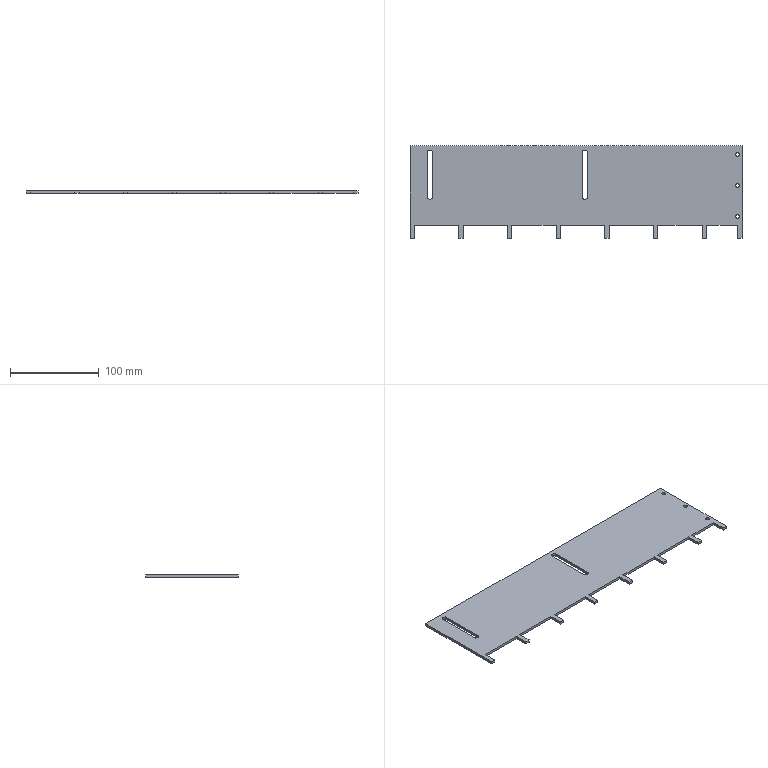Part | SolidWorks | features HoleWzd 2, Cut 1, FlatPattern 1, SMBaseFlange 1, SheetMetal 1 | 1 solid | 48 faces | box 375 x 105 x 3 mm | volume 101027 mm3 | plane 38 | cylinder 10 | commonest cylinder face diameters 4.2 x6 5.8 x4
STEP:
#1=CARTESIAN_POINT('',(372.1,60.,0.));
#2=VERTEX_POINT('',#1);
#3=CARTESIAN_POINT('',(367.9,60.,0.));
#4=VERTEX_POINT('',#3);
#5=CARTESIAN_POINT('',(370.,60.,0.));
#6=DIRECTION('',(0.,0.,-1.));
#7=DIRECTION('',(-1.,0.,0.));
#8=AXIS2_PLACEMENT_3D('',#5,#6,#7);
#9=CIRCLE('',#8,2.1);
#10=EDGE_CURVE('',#2,#4,#9,.T.);
#11=ORIENTED_EDGE('',*,*,#10,.F.);
#12=CARTESIAN_POINT('',(372.1,60.,-3.));
#13=VERTEX_POINT('',#12);
#14=CARTESIAN_POINT('',(372.1,60.,-3.));
#15=DIRECTION('',(0.,0.,-1.));
#16=VECTOR('',#15,1000.);
#17=LINE('',#14,#16);
#18=EDGE_CURVE('',#2,#13,#17,.T.);
#19=ORIENTED_EDGE('',*,*,#18,.T.);
#20=CARTESIAN_POINT('',(367.9,60.,-3.));
#21=VERTEX_POINT('',#20);
#22=CARTESIAN_POINT('',(370.,60.,-3.));
#23=DIRECTION('',(0.,0.,-1.));
#24=DIRECTION('',(-1.,0.,0.));
#25=AXIS2_PLACEMENT_3D('',#22,#23,#24);
#26=CIRCLE('',#25,2.1);
#27=EDGE_CURVE('',#13,#21,#26,.T.);
#28=ORIENTED_EDGE('',*,*,#27,.T.);
#29=CARTESIAN_POINT('',(367.9,60.,-3.));
#30=DIRECTION('',(0.,0.,-1.));
#31=VECTOR('',#30,1000.);
#32=LINE('',#29,#31);
#33=EDGE_CURVE('',#4,#21,#32,.T.);
#34=ORIENTED_EDGE('',*,*,#33,.F.);
#35=EDGE_LOOP('',(#11,#19,#28,#34));
#36=FACE_OUTER_BOUND('',#35,.T.);
#37=CARTESIAN_POINT('',(370.,60.,-3.));
#38=DIRECTION('',(0.,0.,-1.));
#39=DIRECTION('',(-1.,0.,0.));
#40=AXIS2_PLACEMENT_3D('',#37,#38,#39);
#41=CYLINDRICAL_SURFACE('',#40,2.1);
#42=ADVANCED_FACE('',(#36),#41,.F.);
#43=CARTESIAN_POINT('',(372.1,95.,0.));
#44=VERTEX_POINT('',#43);
#45=CARTESIAN_POINT('',(367.9,95.,0.));
#46=VERTEX_POINT('',#45);
#47=CARTESIAN_POINT('',(370.,95.,0.));
#48=DIRECTION('',(0.,0.,-1.));
#49=DIRECTION('',(-1.,0.,0.));
#50=AXIS2_PLACEMENT_3D('',#47,#48,#49);
#51=CIRCLE('',#50,2.1);
#52=EDGE_CURVE('',#44,#46,#51,.T.);
#53=ORIENTED_EDGE('',*,*,#52,.F.);
#54=CARTESIAN_POINT('',(372.1,95.,-3.));
#55=VERTEX_POINT('',#54);
#56=CARTESIAN_POINT('',(372.1,95.,-3.));
#57=DIRECTION('',(0.,0.,-1.));
#58=VECTOR('',#57,1000.);
#59=LINE('',#56,#58);
#60=EDGE_CURVE('',#44,#55,#59,.T.);
#61=ORIENTED_EDGE('',*,*,#60,.T.);
#62=CARTESIAN_POINT('',(367.9,95.,-3.));
#63=VERTEX_POINT('',#62);
#64=CARTESIAN_POINT('',(370.,95.,-3.));
#65=DIRECTION('',(0.,0.,-1.));
#66=DIRECTION('',(-1.,0.,0.));
#67=AXIS2_PLACEMENT_3D('',#64,#65,#66);
#68=CIRCLE('',#67,2.1);
#69=EDGE_CURVE('',#55,#63,#68,.T.);
#70=ORIENTED_EDGE('',*,*,#69,.T.);
#71=CARTESIAN_POINT('',(367.9,95.,-3.));
#72=DIRECTION('',(0.,0.,-1.));
#73=VECTOR('',#72,1000.);
#74=LINE('',#71,#73);
#75=EDGE_CURVE('',#46,#63,#74,.T.);
#76=ORIENTED_EDGE('',*,*,#75,.F.);
#77=EDGE_LOOP('',(#53,#61,#70,#76));
#78=FACE_OUTER_BOUND('',#77,.T.);
#79=CARTESIAN_POINT('',(370.,95.,-3.));
#80=DIRECTION('',(0.,0.,-1.));
#81=DIRECTION('',(-1.,0.,0.));
#82=AXIS2_PLACEMENT_3D('',#79,#80,#81);
#83=CYLINDRICAL_SURFACE('',#82,2.1);
#84=ADVANCED_FACE('',(#78),#83,.F.);
#85=CARTESIAN_POINT('',(372.1,25.,0.));
#86=VERTEX_POINT('',#85);
#87=CARTESIAN_POINT('',(367.9,25.,0.));
#88=VERTEX_POINT('',#87);
#89=CARTESIAN_POINT('',(370.,25.,0.));
#90=DIRECTION('',(0.,0.,-1.));
#91=DIRECTION('',(-1.,0.,0.));
#92=AXIS2_PLACEMENT_3D('',#89,#90,#91);
#93=CIRCLE('',#92,2.1);
#94=EDGE_CURVE('',#86,#88,#93,.T.);
#95=ORIENTED_EDGE('',*,*,#94,.F.);
#96=CARTESIAN_POINT('',(372.1,25.,-3.));
#97=VERTEX_POINT('',#96);
#98=CARTESIAN_POINT('',(372.1,25.,-3.));
#99=DIRECTION('',(0.,0.,-1.));
#100=VECTOR('',#99,1000.);
#101=LINE('',#98,#100);
#102=EDGE_CURVE('',#86,#97,#101,.T.);
#103=ORIENTED_EDGE('',*,*,#102,.T.);
#104=CARTESIAN_POINT('',(367.9,25.,-3.));
#105=VERTEX_POINT('',#104);
#106=CARTESIAN_POINT('',(370.,25.,-3.));
#107=DIRECTION('',(0.,0.,-1.));
#108=DIRECTION('',(-1.,0.,0.));
#109=AXIS2_PLACEMENT_3D('',#106,#107,#108);
#110=CIRCLE('',#109,2.1);
#111=EDGE_CURVE('',#97,#105,#110,.T.);
#112=ORIENTED_EDGE('',*,*,#111,.T.);
#113=CARTESIAN_POINT('',(367.9,25.,-3.));
#114=DIRECTION('',(0.,0.,-1.));
#115=VECTOR('',#114,1000.);
#116=LINE('',#113,#115);
#117=EDGE_CURVE('',#88,#105,#116,.T.);
#118=ORIENTED_EDGE('',*,*,#117,.F.);
#119=EDGE_LOOP('',(#95,#103,#112,#118));
#120=FACE_OUTER_BOUND('',#119,.T.);
#121=CARTESIAN_POINT('',(370.,25.,-3.));
#122=DIRECTION('',(0.,0.,-1.));
#123=DIRECTION('',(-1.,0.,0.));
#124=AXIS2_PLACEMENT_3D('',#121,#122,#123);
#125=CYLINDRICAL_SURFACE('',#124,2.1);
#126=ADVANCED_FACE('',(#120),#125,.F.);
#127=CARTESIAN_POINT('',(5.,0.,-3.));
#128=VERTEX_POINT('',#127);
#129=CARTESIAN_POINT('',(5.,0.,0.));
#130=VERTEX_POINT('',#129);
#131=CARTESIAN_POINT('',(5.,0.,-3.));
#132=DIRECTION('',(0.,0.,1.));
#133=VECTOR('',#132,1000.);
#134=LINE('',#131,#133);
#135=EDGE_CURVE('',#128,#130,#134,.T.);
#136=ORIENTED_EDGE('',*,*,#135,.T.);
#137=CARTESIAN_POINT('',(0.,0.,0.));
#138=VERTEX_POINT('',#137);
#139=CARTESIAN_POINT('',(0.,0.,0.));
#140=DIRECTION('',(1.,0.,0.));
#141=VECTOR('',#140,1000.);
#142=LINE('',#139,#141);
#143=EDGE_CURVE('',#138,#130,#142,.T.);
#144=ORIENTED_EDGE('',*,*,#143,.F.);
#145=CARTESIAN_POINT('',(0.,0.,-3.));
#146=VERTEX_POINT('',#145);
#147=CARTESIAN_POINT('',(0.,0.,-3.));
#148=DIRECTION('',(0.,0.,1.));
#149=VECTOR('',#148,1000.);
#150=LINE('',#147,#149);
#151=EDGE_CURVE('',#146,#138,#150,.T.);
#152=ORIENTED_EDGE('',*,*,#151,.F.);
#153=CARTESIAN_POINT('',(0.,0.,-3.));
#154=DIRECTION('',(1.,0.,0.));
#155=VECTOR('',#154,1000.);
#156=LINE('',#153,#155);
#157=EDGE_CURVE('',#146,#128,#156,.T.);
#158=ORIENTED_EDGE('',*,*,#157,.T.);
#159=EDGE_LOOP('',(#136,#144,#152,#158));
#160=FACE_OUTER_BOUND('',#159,.T.);
#161=CARTESIAN_POINT('',(0.,0.,-3.));
#162=DIRECTION('',(0.,-1.,0.));
#163=DIRECTION('',(0.,0.,-1.));
#164=AXIS2_PLACEMENT_3D('',#161,#162,#163);
#165=PLANE('',#164);
#166=ADVANCED_FACE('',(#160),#165,.T.);
#167=CARTESIAN_POINT('',(280.,0.,-3.));
#168=VERTEX_POINT('',#167);
#169=CARTESIAN_POINT('',(280.,0.,0.));
#170=VERTEX_POINT('',#169);
#171=CARTESIAN_POINT('',(280.,0.,-3.));
#172=DIRECTION('',(0.,0.,1.));
#173=VECTOR('',#172,1000.);
#174=LINE('',#171,#173);
#175=EDGE_CURVE('',#168,#170,#174,.T.);
#176=ORIENTED_EDGE('',*,*,#175,.T.);
#177=CARTESIAN_POINT('',(275.,0.,0.));
#178=VERTEX_POINT('',#177);
#179=CARTESIAN_POINT('',(0.,0.,0.));
#180=DIRECTION('',(1.,0.,0.));
#181=VECTOR('',#180,1000.);
#182=LINE('',#179,#181);
#183=EDGE_CURVE('',#178,#170,#182,.T.);
#184=ORIENTED_EDGE('',*,*,#183,.F.);
#185=CARTESIAN_POINT('',(275.,0.,-3.));
#186=VERTEX_POINT('',#185);
#187=CARTESIAN_POINT('',(275.,0.,-3.));
#188=DIRECTION('',(0.,0.,1.));
#189=VECTOR('',#188,1000.);
#190=LINE('',#187,#189);
#191=EDGE_CURVE('',#186,#178,#190,.T.);
#192=ORIENTED_EDGE('',*,*,#191,.F.);
#193=CARTESIAN_POINT('',(0.,0.,-3.));
#194=DIRECTION('',(1.,0.,0.));
#195=VECTOR('',#194,1000.);
#196=LINE('',#193,#195);
#197=EDGE_CURVE('',#186,#168,#196,.T.);
#198=ORIENTED_EDGE('',*,*,#197,.T.);
#199=EDGE_LOOP('',(#176,#184,#192,#198));
#200=FACE_OUTER_BOUND('',#199,.T.);
#201=CARTESIAN_POINT('',(0.,0.,-3.));
#202=DIRECTION('',(0.,-1.,0.));
#203=DIRECTION('',(0.,0.,-1.));
#204=AXIS2_PLACEMENT_3D('',#201,#202,#203);
#205=PLANE('',#204);
#206=ADVANCED_FACE('',(#200),#205,.T.);
#207=CARTESIAN_POINT('',(225.,0.,-3.));
#208=VERTEX_POINT('',#207);
#209=CARTESIAN_POINT('',(225.,0.,0.));
#210=VERTEX_POINT('',#209);
#211=CARTESIAN_POINT('',(225.,0.,-3.));
#212=DIRECTION('',(0.,0.,1.));
#213=VECTOR('',#212,1000.);
#214=LINE('',#211,#213);
#215=EDGE_CURVE('',#208,#210,#214,.T.);
#216=ORIENTED_EDGE('',*,*,#215,.T.);
#217=CARTESIAN_POINT('',(220.,0.,0.));
#218=VERTEX_POINT('',#217);
#219=CARTESIAN_POINT('',(0.,0.,0.));
#220=DIRECTION('',(1.,0.,0.));
#221=VECTOR('',#220,1000.);
#222=LINE('',#219,#221);
#223=EDGE_CURVE('',#218,#210,#222,.T.);
#224=ORIENTED_EDGE('',*,*,#223,.F.);
#225=CARTESIAN_POINT('',(220.,0.,-3.));
#226=VERTEX_POINT('',#225);
#227=CARTESIAN_POINT('',(220.,0.,-3.));
#228=DIRECTION('',(0.,0.,1.));
#229=VECTOR('',#228,1000.);
#230=LINE('',#227,#229);
#231=EDGE_CURVE('',#226,#218,#230,.T.);
#232=ORIENTED_EDGE('',*,*,#231,.F.);
#233=CARTESIAN_POINT('',(0.,0.,-3.));
#234=DIRECTION('',(1.,0.,0.));
#235=VECTOR('',#234,1000.);
#236=LINE('',#233,#235);
#237=EDGE_CURVE('',#226,#208,#236,.T.);
#238=ORIENTED_EDGE('',*,*,#237,.T.);
#239=EDGE_LOOP('',(#216,#224,#232,#238));
#240=FACE_OUTER_BOUND('',#239,.T.);
#241=CARTESIAN_POINT('',(0.,0.,-3.));
#242=DIRECTION('',(0.,-1.,0.));
#243=DIRECTION('',(0.,0.,-1.));
#244=AXIS2_PLACEMENT_3D('',#241,#242,#243);
#245=PLANE('',#244);
#246=ADVANCED_FACE('',(#240),#245,.T.);
#247=CARTESIAN_POINT('',(330.,0.,-3.));
#248=VERTEX_POINT('',#247);
#249=CARTESIAN_POINT('',(330.,0.,0.));
#250=VERTEX_POINT('',#249);
#251=CARTESIAN_POINT('',(330.,0.,-3.));
#252=DIRECTION('',(0.,0.,1.));
#253=VECTOR('',#252,1000.);
#254=LINE('',#251,#253);
#255=EDGE_CURVE('',#248,#250,#254,.T.);
#256=ORIENTED_EDGE('',*,*,#255,.F.);
#257=CARTESIAN_POINT('',(335.,0.,-3.));
#258=VERTEX_POINT('',#257);
#259=CARTESIAN_POINT('',(0.,0.,-3.));
#260=DIRECTION('',(1.,0.,0.));
#261=VECTOR('',#260,1000.);
#262=LINE('',#259,#261);
#263=EDGE_CURVE('',#248,#258,#262,.T.);
#264=ORIENTED_EDGE('',*,*,#263,.T.);
#265=CARTESIAN_POINT('',(335.,0.,0.));
#266=VERTEX_POINT('',#265);
#267=CARTESIAN_POINT('',(335.,0.,-3.));
#268=DIRECTION('',(0.,0.,1.));
#269=VECTOR('',#268,1000.);
#270=LINE('',#267,#269);
#271=EDGE_CURVE('',#258,#266,#270,.T.);
#272=ORIENTED_EDGE('',*,*,#271,.T.);
#273=CARTESIAN_POINT('',(0.,0.,0.));
#274=DIRECTION('',(1.,0.,0.));
#275=VECTOR('',#274,1000.);
#276=LINE('',#273,#275);
#277=EDGE_CURVE('',#250,#266,#276,.T.);
#278=ORIENTED_EDGE('',*,*,#277,.F.);
#279=EDGE_LOOP('',(#256,#264,#272,#278));
#280=FACE_OUTER_BOUND('',#279,.T.);
#281=CARTESIAN_POINT('',(0.,0.,-3.));
#282=DIRECTION('',(0.,-1.,0.));
#283=DIRECTION('',(0.,0.,-1.));
#284=AXIS2_PLACEMENT_3D('',#281,#282,#283);
#285=PLANE('',#284);
#286=ADVANCED_FACE('',(#280),#285,.T.);
#287=CARTESIAN_POINT('',(55.,0.,-3.));
#288=VERTEX_POINT('',#287);
#289=CARTESIAN_POINT('',(55.,0.,0.));
#290=VERTEX_POINT('',#289);
#291=CARTESIAN_POINT('',(55.,0.,-3.));
#292=DIRECTION('',(0.,0.,1.));
#293=VECTOR('',#292,1000.);
#294=LINE('',#291,#293);
#295=EDGE_CURVE('',#288,#290,#294,.T.);
#296=ORIENTED_EDGE('',*,*,#295,.F.);
#297=CARTESIAN_POINT('',(60.,0.,-3.));
#298=VERTEX_POINT('',#297);
#299=CARTESIAN_POINT('',(0.,0.,-3.));
#300=DIRECTION('',(1.,0.,0.));
#301=VECTOR('',#300,1000.);
#302=LINE('',#299,#301);
#303=EDGE_CURVE('',#288,#298,#302,.T.);
#304=ORIENTED_EDGE('',*,*,#303,.T.);
#305=CARTESIAN_POINT('',(60.,0.,0.));
#306=VERTEX_POINT('',#305);
#307=CARTESIAN_POINT('',(60.,0.,-3.));
#308=DIRECTION('',(0.,0.,1.));
#309=VECTOR('',#308,1000.);
#310=LINE('',#307,#309);
#311=EDGE_CURVE('',#298,#306,#310,.T.);
#312=ORIENTED_EDGE('',*,*,#311,.T.);
#313=CARTESIAN_POINT('',(0.,0.,0.));
#314=DIRECTION('',(1.,0.,0.));
#315=VECTOR('',#314,1000.);
#316=LINE('',#313,#315);
#317=EDGE_CURVE('',#290,#306,#316,.T.);
#318=ORIENTED_EDGE('',*,*,#317,.F.);
#319=EDGE_LOOP('',(#296,#304,#312,#318));
#320=FACE_OUTER_BOUND('',#319,.T.);
#321=CARTESIAN_POINT('',(0.,0.,-3.));
#322=DIRECTION('',(0.,-1.,0.));
#323=DIRECTION('',(0.,0.,-1.));
#324=AXIS2_PLACEMENT_3D('',#321,#322,#323);
#325=PLANE('',#324);
#326=ADVANCED_FACE('',(#320),#325,.T.);
#327=CARTESIAN_POINT('',(110.,0.,-3.));
#328=VERTEX_POINT('',#327);
#329=CARTESIAN_POINT('',(110.,0.,0.));
#330=VERTEX_POINT('',#329);
#331=CARTESIAN_POINT('',(110.,0.,-3.));
#332=DIRECTION('',(0.,0.,1.));
#333=VECTOR('',#332,1000.);
#334=LINE('',#331,#333);
#335=EDGE_CURVE('',#328,#330,#334,.T.);
#336=ORIENTED_EDGE('',*,*,#335,.F.);
#337=CARTESIAN_POINT('',(115.,0.,-3.));
#338=VERTEX_POINT('',#337);
#339=CARTESIAN_POINT('',(0.,0.,-3.));
#340=DIRECTION('',(1.,0.,0.));
#341=VECTOR('',#340,1000.);
#342=LINE('',#339,#341);
#343=EDGE_CURVE('',#328,#338,#342,.T.);
#344=ORIENTED_EDGE('',*,*,#343,.T.);
#345=CARTESIAN_POINT('',(115.,0.,0.));
#346=VERTEX_POINT('',#345);
#347=CARTESIAN_POINT('',(115.,0.,-3.));
#348=DIRECTION('',(0.,0.,1.));
#349=VECTOR('',#348,1000.);
#350=LINE('',#347,#349);
#351=EDGE_CURVE('',#338,#346,#350,.T.);
#352=ORIENTED_EDGE('',*,*,#351,.T.);
#353=CARTESIAN_POINT('',(0.,0.,0.));
#354=DIRECTION('',(1.,0.,0.));
#355=VECTOR('',#354,1000.);
#356=LINE('',#353,#355);
#357=EDGE_CURVE('',#330,#346,#356,.T.);
#358=ORIENTED_EDGE('',*,*,#357,.F.);
#359=EDGE_LOOP('',(#336,#344,#352,#358));
#360=FACE_OUTER_BOUND('',#359,.T.);
#361=CARTESIAN_POINT('',(0.,0.,-3.));
#362=DIRECTION('',(0.,-1.,0.));
#363=DIRECTION('',(0.,0.,-1.));
#364=AXIS2_PLACEMENT_3D('',#361,#362,#363);
#365=PLANE('',#364);
#366=ADVANCED_FACE('',(#360),#365,.T.);
#367=CARTESIAN_POINT('',(165.,0.,-3.));
#368=VERTEX_POINT('',#367);
#369=CARTESIAN_POINT('',(165.,0.,0.));
#370=VERTEX_POINT('',#369);
#371=CARTESIAN_POINT('',(165.,0.,-3.));
#372=DIRECTION('',(0.,0.,1.));
#373=VECTOR('',#372,1000.);
#374=LINE('',#371,#373);
#375=EDGE_CURVE('',#368,#370,#374,.T.);
#376=ORIENTED_EDGE('',*,*,#375,.F.);
#377=CARTESIAN_POINT('',(170.,0.,-3.));
#378=VERTEX_POINT('',#377);
#379=CARTESIAN_POINT('',(0.,0.,-3.));
#380=DIRECTION('',(1.,0.,0.));
#381=VECTOR('',#380,1000.);
#382=LINE('',#379,#381);
#383=EDGE_CURVE('',#368,#378,#382,.T.);
#384=ORIENTED_EDGE('',*,*,#383,.T.);
#385=CARTESIAN_POINT('',(170.,0.,0.));
#386=VERTEX_POINT('',#385);
#387=CARTESIAN_POINT('',(170.,0.,-3.));
#388=DIRECTION('',(0.,0.,1.));
#389=VECTOR('',#388,1000.);
#390=LINE('',#387,#389);
#391=EDGE_CURVE('',#378,#386,#390,.T.);
#392=ORIENTED_EDGE('',*,*,#391,.T.);
#393=CARTESIAN_POINT('',(0.,0.,0.));
#394=DIRECTION('',(1.,0.,0.));
#395=VECTOR('',#394,1000.);
#396=LINE('',#393,#395);
#397=EDGE_CURVE('',#370,#386,#396,.T.);
#398=ORIENTED_EDGE('',*,*,#397,.F.);
#399=EDGE_LOOP('',(#376,#384,#392,#398));
#400=FACE_OUTER_BOUND('',#399,.T.);
#401=CARTESIAN_POINT('',(0.,0.,-3.));
#402=DIRECTION('',(0.,-1.,0.));
#403=DIRECTION('',(0.,0.,-1.));
#404=AXIS2_PLACEMENT_3D('',#401,#402,#403);
#405=PLANE('',#404);
#406=ADVANCED_FACE('',(#400),#405,.T.);
#407=CARTESIAN_POINT('',(370.,60.,0.));
#408=DIRECTION('',(0.,0.,-1.));
#409=DIRECTION('',(-1.,0.,0.));
#410=AXIS2_PLACEMENT_3D('',#407,#408,#409);
#411=CIRCLE('',#410,2.1);
#412=EDGE_CURVE('',#4,#2,#411,.T.);
#413=ORIENTED_EDGE('',*,*,#412,.T.);
#414=ORIENTED_EDGE('',*,*,#10,.T.);
#415=EDGE_LOOP('',(#413,#414));
#416=FACE_BOUND('',#415,.T.);
#417=CARTESIAN_POINT('',(370.,95.,0.));
#418=DIRECTION('',(0.,0.,-1.));
#419=DIRECTION('',(-1.,0.,0.));
#420=AXIS2_PLACEMENT_3D('',#417,#418,#419);
#421=CIRCLE('',#420,2.1);
#422=EDGE_CURVE('',#46,#44,#421,.T.);
#423=ORIENTED_EDGE('',*,*,#422,.T.);
#424=ORIENTED_EDGE('',*,*,#52,.T.);
#425=EDGE_LOOP('',(#423,#424));
#426=FACE_BOUND('',#425,.T.);
#427=CARTESIAN_POINT('',(370.,25.,0.));
#428=DIRECTION('',(0.,0.,-1.));
#429=DIRECTION('',(-1.,0.,0.));
#430=AXIS2_PLACEMENT_3D('',#427,#428,#429);
#431=CIRCLE('',#430,2.1);
#432=EDGE_CURVE('',#88,#86,#431,.T.);
#433=ORIENTED_EDGE('',*,*,#432,.T.);
#434=ORIENTED_EDGE('',*,*,#94,.T.);
#435=EDGE_LOOP('',(#433,#434));
#436=FACE_BOUND('',#435,.T.);
#437=CARTESIAN_POINT('',(25.4,47.,0.));
#438=VERTEX_POINT('',#437);
#439=CARTESIAN_POINT('',(25.4,97.,0.));
#440=VERTEX_POINT('',#439);
#441=CARTESIAN_POINT('',(25.4,47.,0.));
#442=DIRECTION('',(0.,1.,0.));
#443=VECTOR('',#442,1000.);
#444=LINE('',#441,#443);
#445=EDGE_CURVE('',#438,#440,#444,.T.);
#446=ORIENTED_EDGE('',*,*,#445,.F.);
#447=CARTESIAN_POINT('',(19.6,47.,0.));
#448=VERTEX_POINT('',#447);
#449=CARTESIAN_POINT('',(22.5,47.,0.));
#450=DIRECTION('',(0.,0.,1.));
#451=DIRECTION('',(1.,0.,0.));
#452=AXIS2_PLACEMENT_3D('',#449,#450,#451);
#453=CIRCLE('',#452,2.9);
#454=EDGE_CURVE('',#448,#438,#453,.T.);
#455=ORIENTED_EDGE('',*,*,#454,.F.);
#456=CARTESIAN_POINT('',(19.6,97.,0.));
#457=VERTEX_POINT('',#456);
#458=CARTESIAN_POINT('',(19.6,47.,0.));
#459=DIRECTION('',(0.,1.,0.));
#460=VECTOR('',#459,1000.);
#461=LINE('',#458,#460);
#462=EDGE_CURVE('',#448,#457,#461,.T.);
#463=ORIENTED_EDGE('',*,*,#462,.T.);
#464=CARTESIAN_POINT('',(22.5,97.,0.));
#465=DIRECTION('',(0.,0.,1.));
#466=DIRECTION('',(1.,0.,0.));
#467=AXIS2_PLACEMENT_3D('',#464,#465,#466);
#468=CIRCLE('',#467,2.9);
#469=EDGE_CURVE('',#440,#457,#468,.T.);
#470=ORIENTED_EDGE('',*,*,#469,.F.);
#471=EDGE_LOOP('',(#446,#455,#463,#470));
#472=FACE_BOUND('',#471,.T.);
#473=ORIENTED_EDGE('',*,*,#143,.T.);
#474=CARTESIAN_POINT('',(5.,15.,0.));
#475=VERTEX_POINT('',#474);
#476=CARTESIAN_POINT('',(5.,15.,0.));
#477=DIRECTION('',(0.,-1.,0.));
#478=VECTOR('',#477,1000.);
#479=LINE('',#476,#478);
#480=EDGE_CURVE('',#475,#130,#479,.T.);
#481=ORIENTED_EDGE('',*,*,#480,.F.);
#482=CARTESIAN_POINT('',(55.,15.,0.));
#483=VERTEX_POINT('',#482);
#484=CARTESIAN_POINT('',(5.,15.,0.));
#485=DIRECTION('',(-1.,0.,0.));
#486=VECTOR('',#485,1000.);
#487=LINE('',#484,#486);
#488=EDGE_CURVE('',#483,#475,#487,.T.);
#489=ORIENTED_EDGE('',*,*,#488,.F.);
#490=CARTESIAN_POINT('',(55.,15.,0.));
#491=DIRECTION('',(0.,1.,0.));
#492=VECTOR('',#491,1000.);
#493=LINE('',#490,#492);
#494=EDGE_CURVE('',#290,#483,#493,.T.);
#495=ORIENTED_EDGE('',*,*,#494,.F.);
#496=ORIENTED_EDGE('',*,*,#317,.T.);
#497=CARTESIAN_POINT('',(60.,15.,0.));
#498=VERTEX_POINT('',#497);
#499=CARTESIAN_POINT('',(60.,15.,0.));
#500=DIRECTION('',(0.,-1.,0.));
#501=VECTOR('',#500,1000.);
#502=LINE('',#499,#501);
#503=EDGE_CURVE('',#498,#306,#502,.T.);
#504=ORIENTED_EDGE('',*,*,#503,.F.);
#505=CARTESIAN_POINT('',(110.,15.,0.));
#506=VERTEX_POINT('',#505);
#507=CARTESIAN_POINT('',(60.,15.,0.));
#508=DIRECTION('',(-1.,0.,0.));
#509=VECTOR('',#508,1000.);
#510=LINE('',#507,#509);
#511=EDGE_CURVE('',#506,#498,#510,.T.);
#512=ORIENTED_EDGE('',*,*,#511,.F.);
#513=CARTESIAN_POINT('',(110.,15.,0.));
#514=DIRECTION('',(0.,1.,0.));
#515=VECTOR('',#514,1000.);
#516=LINE('',#513,#515);
#517=EDGE_CURVE('',#330,#506,#516,.T.);
#518=ORIENTED_EDGE('',*,*,#517,.F.);
#519=ORIENTED_EDGE('',*,*,#357,.T.);
#520=CARTESIAN_POINT('',(115.,15.,0.));
#521=VERTEX_POINT('',#520);
#522=CARTESIAN_POINT('',(115.,15.,0.));
#523=DIRECTION('',(0.,-1.,0.));
#524=VECTOR('',#523,1000.);
#525=LINE('',#522,#524);
#526=EDGE_CURVE('',#521,#346,#525,.T.);
#527=ORIENTED_EDGE('',*,*,#526,.F.);
#528=CARTESIAN_POINT('',(165.,15.,0.));
#529=VERTEX_POINT('',#528);
#530=CARTESIAN_POINT('',(115.,15.,0.));
#531=DIRECTION('',(-1.,0.,0.));
#532=VECTOR('',#531,1000.);
#533=LINE('',#530,#532);
#534=EDGE_CURVE('',#529,#521,#533,.T.);
#535=ORIENTED_EDGE('',*,*,#534,.F.);
#536=CARTESIAN_POINT('',(165.,15.,0.));
#537=DIRECTION('',(0.,1.,0.));
#538=VECTOR('',#537,1000.);
#539=LINE('',#536,#538);
#540=EDGE_CURVE('',#370,#529,#539,.T.);
#541=ORIENTED_EDGE('',*,*,#540,.F.);
#542=ORIENTED_EDGE('',*,*,#397,.T.);
#543=CARTESIAN_POINT('',(170.,15.,0.));
#544=VERTEX_POINT('',#543);
#545=CARTESIAN_POINT('',(170.,15.,0.));
#546=DIRECTION('',(0.,-1.,0.));
#547=VECTOR('',#546,1000.);
#548=LINE('',#545,#547);
#549=EDGE_CURVE('',#544,#386,#548,.T.);
#550=ORIENTED_EDGE('',*,*,#549,.F.);
#551=CARTESIAN_POINT('',(220.,15.,0.));
#552=VERTEX_POINT('',#551);
#553=CARTESIAN_POINT('',(170.,15.,0.));
#554=DIRECTION('',(-1.,0.,0.));
#555=VECTOR('',#554,1000.);
#556=LINE('',#553,#555);
#557=EDGE_CURVE('',#552,#544,#556,.T.);
#558=ORIENTED_EDGE('',*,*,#557,.F.);
#559=CARTESIAN_POINT('',(220.,15.,0.));
#560=DIRECTION('',(0.,1.,0.));
#561=VECTOR('',#560,1000.);
#562=LINE('',#559,#561);
#563=EDGE_CURVE('',#218,#552,#562,.T.);
#564=ORIENTED_EDGE('',*,*,#563,.F.);
#565=ORIENTED_EDGE('',*,*,#223,.T.);
#566=CARTESIAN_POINT('',(225.,15.,0.));
#567=VERTEX_POINT('',#566);
#568=CARTESIAN_POINT('',(225.,15.,0.));
#569=DIRECTION('',(0.,-1.,0.));
#570=VECTOR('',#569,1000.);
#571=LINE('',#568,#570);
#572=EDGE_CURVE('',#567,#210,#571,.T.);
#573=ORIENTED_EDGE('',*,*,#572,.F.);
#574=CARTESIAN_POINT('',(275.,15.,0.));
#575=VERTEX_POINT('',#574);
#576=CARTESIAN_POINT('',(225.,15.,0.));
#577=DIRECTION('',(-1.,0.,0.));
#578=VECTOR('',#577,1000.);
#579=LINE('',#576,#578);
#580=EDGE_CURVE('',#575,#567,#579,.T.);
#581=ORIENTED_EDGE('',*,*,#580,.F.);
#582=CARTESIAN_POINT('',(275.,15.,0.));
#583=DIRECTION('',(0.,1.,0.));
#584=VECTOR('',#583,1000.);
#585=LINE('',#582,#584);
#586=EDGE_CURVE('',#178,#575,#585,.T.);
#587=ORIENTED_EDGE('',*,*,#586,.F.);
#588=ORIENTED_EDGE('',*,*,#183,.T.);
#589=CARTESIAN_POINT('',(280.,15.,0.));
#590=VERTEX_POINT('',#589);
#591=CARTESIAN_POINT('',(280.,15.,0.));
#592=DIRECTION('',(0.,-1.,0.));
#593=VECTOR('',#592,1000.);
#594=LINE('',#591,#593);
#595=EDGE_CURVE('',#590,#170,#594,.T.);
#596=ORIENTED_EDGE('',*,*,#595,.F.);
#597=CARTESIAN_POINT('',(330.,15.,0.));
#598=VERTEX_POINT('',#597);
#599=CARTESIAN_POINT('',(280.,15.,0.));
#600=DIRECTION('',(-1.,0.,0.));
#601=VECTOR('',#600,1000.);
#602=LINE('',#599,#601);
#603=EDGE_CURVE('',#598,#590,#602,.T.);
#604=ORIENTED_EDGE('',*,*,#603,.F.);
#605=CARTESIAN_POINT('',(330.,15.,0.));
#606=DIRECTION('',(0.,1.,0.));
#607=VECTOR('',#606,1000.);
#608=LINE('',#605,#607);
#609=EDGE_CURVE('',#250,#598,#608,.T.);
#610=ORIENTED_EDGE('',*,*,#609,.F.);
#611=ORIENTED_EDGE('',*,*,#277,.T.);
#612=CARTESIAN_POINT('',(335.,15.,0.));
#613=VERTEX_POINT('',#612);
#614=CARTESIAN_POINT('',(335.,15.,0.));
#615=DIRECTION('',(0.,-1.,0.));
#616=VECTOR('',#615,1000.);
#617=LINE('',#614,#616);
#618=EDGE_CURVE('',#613,#266,#617,.T.);
#619=ORIENTED_EDGE('',*,*,#618,.F.);
#620=CARTESIAN_POINT('',(370.,15.,0.));
#621=VERTEX_POINT('',#620);
#622=CARTESIAN_POINT('',(335.,15.,0.));
#623=DIRECTION('',(-1.,0.,0.));
#624=VECTOR('',#623,1000.);
#625=LINE('',#622,#624);
#626=EDGE_CURVE('',#621,#613,#625,.T.);
#627=ORIENTED_EDGE('',*,*,#626,.F.);
#628=CARTESIAN_POINT('',(370.,0.,0.));
#629=VERTEX_POINT('',#628);
#630=CARTESIAN_POINT('',(370.,15.,0.));
#631=DIRECTION('',(0.,1.,0.));
#632=VECTOR('',#631,1000.);
#633=LINE('',#630,#632);
#634=EDGE_CURVE('',#629,#621,#633,.T.);
#635=ORIENTED_EDGE('',*,*,#634,.F.);
#636=CARTESIAN_POINT('',(375.,0.,0.));
#637=VERTEX_POINT('',#636);
#638=CARTESIAN_POINT('',(0.,0.,0.));
#639=DIRECTION('',(1.,0.,0.));
#640=VECTOR('',#639,1000.);
#641=LINE('',#638,#640);
#642=EDGE_CURVE('',#629,#637,#641,.T.);
#643=ORIENTED_EDGE('',*,*,#642,.T.);
#644=CARTESIAN_POINT('',(375.,105.,0.));
#645=VERTEX_POINT('',#644);
#646=CARTESIAN_POINT('',(375.,0.,0.));
#647=DIRECTION('',(0.,1.,0.));
#648=VECTOR('',#647,1000.);
#649=LINE('',#646,#648);
#650=EDGE_CURVE('',#637,#645,#649,.T.);
#651=ORIENTED_EDGE('',*,*,#650,.T.);
#652=CARTESIAN_POINT('',(0.,105.,0.));
#653=VERTEX_POINT('',#652);
#654=CARTESIAN_POINT('',(0.,105.,0.));
#655=DIRECTION('',(-1.,0.,0.));
#656=VECTOR('',#655,1000.);
#657=LINE('',#654,#656);
#658=EDGE_CURVE('',#645,#653,#657,.T.);
#659=ORIENTED_EDGE('',*,*,#658,.T.);
#660=CARTESIAN_POINT('',(0.,0.,0.));
#661=DIRECTION('',(0.,-1.,0.));
#662=VECTOR('',#661,1000.);
#663=LINE('',#660,#662);
#664=EDGE_CURVE('',#653,#138,#663,.T.);
#665=ORIENTED_EDGE('',*,*,#664,.T.);
#666=EDGE_LOOP('',(#473,#481,#489,#495,#496,#504,#512,#518,#519,#527,#535,#541,#542,#550,#558,#564,#565,#573,#581,#587,#588,#596,#604,#610,#611,#619,#627,#635,#643,#651,#659,#665));
#667=FACE_OUTER_BOUND('',#666,.T.);
#668=CARTESIAN_POINT('',(200.4,47.,0.));
#669=VERTEX_POINT('',#668);
#670=CARTESIAN_POINT('',(200.4,97.,0.));
#671=VERTEX_POINT('',#670);
#672=CARTESIAN_POINT('',(200.4,47.,0.));
#673=DIRECTION('',(0.,1.,0.));
#674=VECTOR('',#673,1000.);
#675=LINE('',#672,#674);
#676=EDGE_CURVE('',#669,#671,#675,.T.);
#677=ORIENTED_EDGE('',*,*,#676,.F.);
#678=CARTESIAN_POINT('',(194.6,47.,0.));
#679=VERTEX_POINT('',#678);
#680=CARTESIAN_POINT('',(197.5,47.,0.));
#681=DIRECTION('',(0.,0.,1.));
#682=DIRECTION('',(1.,0.,0.));
#683=AXIS2_PLACEMENT_3D('',#680,#681,#682);
#684=CIRCLE('',#683,2.9);
#685=EDGE_CURVE('',#679,#669,#684,.T.);
#686=ORIENTED_EDGE('',*,*,#685,.F.);
#687=CARTESIAN_POINT('',(194.6,97.,0.));
#688=VERTEX_POINT('',#687);
#689=CARTESIAN_POINT('',(194.6,47.,0.));
#690=DIRECTION('',(0.,1.,0.));
#691=VECTOR('',#690,1000.);
#692=LINE('',#689,#691);
#693=EDGE_CURVE('',#679,#688,#692,.T.);
#694=ORIENTED_EDGE('',*,*,#693,.T.);
#695=CARTESIAN_POINT('',(197.5,97.,0.));
#696=DIRECTION('',(0.,0.,1.));
#697=DIRECTION('',(1.,0.,0.));
#698=AXIS2_PLACEMENT_3D('',#695,#696,#697);
#699=CIRCLE('',#698,2.9);
#700=EDGE_CURVE('',#671,#688,#699,.T.);
#701=ORIENTED_EDGE('',*,*,#700,.F.);
#702=EDGE_LOOP('',(#677,#686,#694,#701));
#703=FACE_BOUND('',#702,.T.);
#704=CARTESIAN_POINT('',(0.,0.,0.));
#705=DIRECTION('',(0.,0.,-1.));
#706=DIRECTION('',(-1.,0.,0.));
#707=AXIS2_PLACEMENT_3D('',#704,#705,#706);
#708=PLANE('',#707);
#709=ADVANCED_FACE('',(#416,#426,#436,#472,#667,#703),#708,.F.);
#710=ORIENTED_EDGE('',*,*,#664,.F.);
#711=CARTESIAN_POINT('',(0.,105.,-3.));
#712=VERTEX_POINT('',#711);
#713=CARTESIAN_POINT('',(0.,105.,-3.));
#714=DIRECTION('',(0.,0.,1.));
#715=VECTOR('',#714,1000.);
#716=LINE('',#713,#715);
#717=EDGE_CURVE('',#712,#653,#716,.T.);
#718=ORIENTED_EDGE('',*,*,#717,.F.);
#719=CARTESIAN_POINT('',(0.,0.,-3.));
#720=DIRECTION('',(0.,-1.,0.));
#721=VECTOR('',#720,1000.);
#722=LINE('',#719,#721);
#723=EDGE_CURVE('',#712,#146,#722,.T.);
#724=ORIENTED_EDGE('',*,*,#723,.T.);
#725=ORIENTED_EDGE('',*,*,#151,.T.);
#726=EDGE_LOOP('',(#710,#718,#724,#725));
#727=FACE_OUTER_BOUND('',#726,.T.);
#728=CARTESIAN_POINT('',(0.,0.,-3.));
#729=DIRECTION('',(-1.,0.,0.));
#730=DIRECTION('',(0.,0.,1.));
#731=AXIS2_PLACEMENT_3D('',#728,#729,#730);
#732=PLANE('',#731);
#733=ADVANCED_FACE('',(#727),#732,.T.);
#734=ORIENTED_EDGE('',*,*,#658,.F.);
#735=CARTESIAN_POINT('',(375.,105.,-3.));
#736=VERTEX_POINT('',#735);
#737=CARTESIAN_POINT('',(375.,105.,-3.));
#738=DIRECTION('',(0.,0.,1.));
#739=VECTOR('',#738,1000.);
#740=LINE('',#737,#739);
#741=EDGE_CURVE('',#736,#645,#740,.T.);
#742=ORIENTED_EDGE('',*,*,#741,.F.);
#743=CARTESIAN_POINT('',(0.,105.,-3.));
#744=DIRECTION('',(-1.,0.,0.));
#745=VECTOR('',#744,1000.);
#746=LINE('',#743,#745);
#747=EDGE_CURVE('',#736,#712,#746,.T.);
#748=ORIENTED_EDGE('',*,*,#747,.T.);
#749=ORIENTED_EDGE('',*,*,#717,.T.);
#750=EDGE_LOOP('',(#734,#742,#748,#749));
#751=FACE_OUTER_BOUND('',#750,.T.);
#752=CARTESIAN_POINT('',(0.,105.,-3.));
#753=DIRECTION('',(0.,1.,0.));
#754=DIRECTION('',(0.,0.,1.));
#755=AXIS2_PLACEMENT_3D('',#752,#753,#754);
#756=PLANE('',#755);
#757=ADVANCED_FACE('',(#751),#756,.T.);
#758=ORIENTED_EDGE('',*,*,#650,.F.);
#759=CARTESIAN_POINT('',(375.,0.,-3.));
#760=VERTEX_POINT('',#759);
#761=CARTESIAN_POINT('',(375.,0.,-3.));
#762=DIRECTION('',(0.,0.,1.));
#763=VECTOR('',#762,1000.);
#764=LINE('',#761,#763);
#765=EDGE_CURVE('',#760,#637,#764,.T.);
#766=ORIENTED_EDGE('',*,*,#765,.F.);
#767=CARTESIAN_POINT('',(375.,0.,-3.));
#768=DIRECTION('',(0.,1.,0.));
#769=VECTOR('',#768,1000.);
#770=LINE('',#767,#769);
#771=EDGE_CURVE('',#760,#736,#770,.T.);
#772=ORIENTED_EDGE('',*,*,#771,.T.);
#773=ORIENTED_EDGE('',*,*,#741,.T.);
#774=EDGE_LOOP('',(#758,#766,#772,#773));
#775=FACE_OUTER_BOUND('',#774,.T.);
#776=CARTESIAN_POINT('',(375.,0.,-3.));
#777=DIRECTION('',(1.,0.,0.));
#778=DIRECTION('',(0.,0.,-1.));
#779=AXIS2_PLACEMENT_3D('',#776,#777,#778);
#780=PLANE('',#779);
#781=ADVANCED_FACE('',(#775),#780,.T.);
#782=CARTESIAN_POINT('',(370.,0.,-3.));
#783=VERTEX_POINT('',#782);
#784=CARTESIAN_POINT('',(370.,0.,-3.));
#785=DIRECTION('',(0.,0.,1.));
#786=VECTOR('',#785,1000.);
#787=LINE('',#784,#786);
#788=EDGE_CURVE('',#783,#629,#787,.T.);
#789=ORIENTED_EDGE('',*,*,#788,.F.);
#790=CARTESIAN_POINT('',(0.,0.,-3.));
#791=DIRECTION('',(1.,0.,0.));
#792=VECTOR('',#791,1000.);
#793=LINE('',#790,#792);
#794=EDGE_CURVE('',#783,#760,#793,.T.);
#795=ORIENTED_EDGE('',*,*,#794,.T.);
#796=ORIENTED_EDGE('',*,*,#765,.T.);
#797=ORIENTED_EDGE('',*,*,#642,.F.);
#798=EDGE_LOOP('',(#789,#795,#796,#797));
#799=FACE_OUTER_BOUND('',#798,.T.);
#800=CARTESIAN_POINT('',(0.,0.,-3.));
#801=DIRECTION('',(0.,-1.,0.));
#802=DIRECTION('',(0.,0.,-1.));
#803=AXIS2_PLACEMENT_3D('',#800,#801,#802);
#804=PLANE('',#803);
#805=ADVANCED_FACE('',(#799),#804,.T.);
#806=CARTESIAN_POINT('',(370.,60.,-3.));
#807=DIRECTION('',(0.,0.,-1.));
#808=DIRECTION('',(-1.,0.,0.));
#809=AXIS2_PLACEMENT_3D('',#806,#807,#808);
#810=CIRCLE('',#809,2.1);
#811=EDGE_CURVE('',#21,#13,#810,.T.);
#812=ORIENTED_EDGE('',*,*,#811,.F.);
#813=ORIENTED_EDGE('',*,*,#27,.F.);
#814=EDGE_LOOP('',(#812,#813));
#815=FACE_BOUND('',#814,.T.);
#816=CARTESIAN_POINT('',(370.,95.,-3.));
#817=DIRECTION('',(0.,0.,-1.));
#818=DIRECTION('',(-1.,0.,0.));
#819=AXIS2_PLACEMENT_3D('',#816,#817,#818);
#820=CIRCLE('',#819,2.1);
#821=EDGE_CURVE('',#63,#55,#820,.T.);
#822=ORIENTED_EDGE('',*,*,#821,.F.);
#823=ORIENTED_EDGE('',*,*,#69,.F.);
#824=EDGE_LOOP('',(#822,#823));
#825=FACE_BOUND('',#824,.T.);
#826=CARTESIAN_POINT('',(370.,25.,-3.));
#827=DIRECTION('',(0.,0.,-1.));
#828=DIRECTION('',(-1.,0.,0.));
#829=AXIS2_PLACEMENT_3D('',#826,#827,#828);
#830=CIRCLE('',#829,2.1);
#831=EDGE_CURVE('',#105,#97,#830,.T.);
#832=ORIENTED_EDGE('',*,*,#831,.F.);
#833=ORIENTED_EDGE('',*,*,#111,.F.);
#834=EDGE_LOOP('',(#832,#833));
#835=FACE_BOUND('',#834,.T.);
#836=CARTESIAN_POINT('',(5.,15.,-3.));
#837=VERTEX_POINT('',#836);
#838=CARTESIAN_POINT('',(5.,15.,-3.));
#839=DIRECTION('',(0.,-1.,0.));
#840=VECTOR('',#839,1000.);
#841=LINE('',#838,#840);
#842=EDGE_CURVE('',#837,#128,#841,.T.);
#843=ORIENTED_EDGE('',*,*,#842,.T.);
#844=ORIENTED_EDGE('',*,*,#157,.F.);
#845=ORIENTED_EDGE('',*,*,#723,.F.);
#846=ORIENTED_EDGE('',*,*,#747,.F.);
#847=ORIENTED_EDGE('',*,*,#771,.F.);
#848=ORIENTED_EDGE('',*,*,#794,.F.);
#849=CARTESIAN_POINT('',(370.,15.,-3.));
#850=VERTEX_POINT('',#849);
#851=CARTESIAN_POINT('',(370.,15.,-3.));
#852=DIRECTION('',(0.,1.,0.));
#853=VECTOR('',#852,1000.);
#854=LINE('',#851,#853);
#855=EDGE_CURVE('',#783,#850,#854,.T.);
#856=ORIENTED_EDGE('',*,*,#855,.T.);
#857=CARTESIAN_POINT('',(335.,15.,-3.));
#858=VERTEX_POINT('',#857);
#859=CARTESIAN_POINT('',(335.,15.,-3.));
#860=DIRECTION('',(-1.,0.,0.));
#861=VECTOR('',#860,1000.);
#862=LINE('',#859,#861);
#863=EDGE_CURVE('',#850,#858,#862,.T.);
#864=ORIENTED_EDGE('',*,*,#863,.T.);
#865=CARTESIAN_POINT('',(335.,15.,-3.));
#866=DIRECTION('',(0.,-1.,0.));
#867=VECTOR('',#866,1000.);
#868=LINE('',#865,#867);
#869=EDGE_CURVE('',#858,#258,#868,.T.);
#870=ORIENTED_EDGE('',*,*,#869,.T.);
#871=ORIENTED_EDGE('',*,*,#263,.F.);
#872=CARTESIAN_POINT('',(330.,15.,-3.));
#873=VERTEX_POINT('',#872);
#874=CARTESIAN_POINT('',(330.,15.,-3.));
#875=DIRECTION('',(0.,1.,0.));
#876=VECTOR('',#875,1000.);
#877=LINE('',#874,#876);
#878=EDGE_CURVE('',#248,#873,#877,.T.);
#879=ORIENTED_EDGE('',*,*,#878,.T.);
#880=CARTESIAN_POINT('',(280.,15.,-3.));
#881=VERTEX_POINT('',#880);
#882=CARTESIAN_POINT('',(280.,15.,-3.));
#883=DIRECTION('',(-1.,0.,0.));
#884=VECTOR('',#883,1000.);
#885=LINE('',#882,#884);
#886=EDGE_CURVE('',#873,#881,#885,.T.);
#887=ORIENTED_EDGE('',*,*,#886,.T.);
#888=CARTESIAN_POINT('',(280.,15.,-3.));
#889=DIRECTION('',(0.,-1.,0.));
#890=VECTOR('',#889,1000.);
#891=LINE('',#888,#890);
#892=EDGE_CURVE('',#881,#168,#891,.T.);
#893=ORIENTED_EDGE('',*,*,#892,.T.);
#894=ORIENTED_EDGE('',*,*,#197,.F.);
#895=CARTESIAN_POINT('',(275.,15.,-3.));
#896=VERTEX_POINT('',#895);
#897=CARTESIAN_POINT('',(275.,15.,-3.));
#898=DIRECTION('',(0.,1.,0.));
#899=VECTOR('',#898,1000.);
#900=LINE('',#897,#899);
#901=EDGE_CURVE('',#186,#896,#900,.T.);
#902=ORIENTED_EDGE('',*,*,#901,.T.);
#903=CARTESIAN_POINT('',(225.,15.,-3.));
#904=VERTEX_POINT('',#903);
#905=CARTESIAN_POINT('',(225.,15.,-3.));
#906=DIRECTION('',(-1.,0.,0.));
#907=VECTOR('',#906,1000.);
#908=LINE('',#905,#907);
#909=EDGE_CURVE('',#896,#904,#908,.T.);
#910=ORIENTED_EDGE('',*,*,#909,.T.);
#911=CARTESIAN_POINT('',(225.,15.,-3.));
#912=DIRECTION('',(0.,-1.,0.));
#913=VECTOR('',#912,1000.);
#914=LINE('',#911,#913);
#915=EDGE_CURVE('',#904,#208,#914,.T.);
#916=ORIENTED_EDGE('',*,*,#915,.T.);
#917=ORIENTED_EDGE('',*,*,#237,.F.);
#918=CARTESIAN_POINT('',(220.,15.,-3.));
#919=VERTEX_POINT('',#918);
#920=CARTESIAN_POINT('',(220.,15.,-3.));
#921=DIRECTION('',(0.,1.,0.));
#922=VECTOR('',#921,1000.);
#923=LINE('',#920,#922);
#924=EDGE_CURVE('',#226,#919,#923,.T.);
#925=ORIENTED_EDGE('',*,*,#924,.T.);
#926=CARTESIAN_POINT('',(170.,15.,-3.));
#927=VERTEX_POINT('',#926);
#928=CARTESIAN_POINT('',(170.,15.,-3.));
#929=DIRECTION('',(-1.,0.,0.));
#930=VECTOR('',#929,1000.);
#931=LINE('',#928,#930);
#932=EDGE_CURVE('',#919,#927,#931,.T.);
#933=ORIENTED_EDGE('',*,*,#932,.T.);
#934=CARTESIAN_POINT('',(170.,15.,-3.));
#935=DIRECTION('',(0.,-1.,0.));
#936=VECTOR('',#935,1000.);
#937=LINE('',#934,#936);
#938=EDGE_CURVE('',#927,#378,#937,.T.);
#939=ORIENTED_EDGE('',*,*,#938,.T.);
#940=ORIENTED_EDGE('',*,*,#383,.F.);
#941=CARTESIAN_POINT('',(165.,15.,-3.));
#942=VERTEX_POINT('',#941);
#943=CARTESIAN_POINT('',(165.,15.,-3.));
#944=DIRECTION('',(0.,1.,0.));
#945=VECTOR('',#944,1000.);
#946=LINE('',#943,#945);
#947=EDGE_CURVE('',#368,#942,#946,.T.);
#948=ORIENTED_EDGE('',*,*,#947,.T.);
#949=CARTESIAN_POINT('',(115.,15.,-3.));
#950=VERTEX_POINT('',#949);
#951=CARTESIAN_POINT('',(115.,15.,-3.));
#952=DIRECTION('',(-1.,0.,0.));
#953=VECTOR('',#952,1000.);
#954=LINE('',#951,#953);
#955=EDGE_CURVE('',#942,#950,#954,.T.);
#956=ORIENTED_EDGE('',*,*,#955,.T.);
#957=CARTESIAN_POINT('',(115.,15.,-3.));
#958=DIRECTION('',(0.,-1.,0.));
#959=VECTOR('',#958,1000.);
#960=LINE('',#957,#959);
#961=EDGE_CURVE('',#950,#338,#960,.T.);
#962=ORIENTED_EDGE('',*,*,#961,.T.);
#963=ORIENTED_EDGE('',*,*,#343,.F.);
#964=CARTESIAN_POINT('',(110.,15.,-3.));
#965=VERTEX_POINT('',#964);
#966=CARTESIAN_POINT('',(110.,15.,-3.));
#967=DIRECTION('',(0.,1.,0.));
#968=VECTOR('',#967,1000.);
#969=LINE('',#966,#968);
#970=EDGE_CURVE('',#328,#965,#969,.T.);
#971=ORIENTED_EDGE('',*,*,#970,.T.);
#972=CARTESIAN_POINT('',(60.,15.,-3.));
#973=VERTEX_POINT('',#972);
#974=CARTESIAN_POINT('',(60.,15.,-3.));
#975=DIRECTION('',(-1.,0.,0.));
#976=VECTOR('',#975,1000.);
#977=LINE('',#974,#976);
#978=EDGE_CURVE('',#965,#973,#977,.T.);
#979=ORIENTED_EDGE('',*,*,#978,.T.);
#980=CARTESIAN_POINT('',(60.,15.,-3.));
#981=DIRECTION('',(0.,-1.,0.));
#982=VECTOR('',#981,1000.);
#983=LINE('',#980,#982);
#984=EDGE_CURVE('',#973,#298,#983,.T.);
#985=ORIENTED_EDGE('',*,*,#984,.T.);
#986=ORIENTED_EDGE('',*,*,#303,.F.);
#987=CARTESIAN_POINT('',(55.,15.,-3.));
#988=VERTEX_POINT('',#987);
#989=CARTESIAN_POINT('',(55.,15.,-3.));
#990=DIRECTION('',(0.,1.,0.));
#991=VECTOR('',#990,1000.);
#992=LINE('',#989,#991);
#993=EDGE_CURVE('',#288,#988,#992,.T.);
#994=ORIENTED_EDGE('',*,*,#993,.T.);
#995=CARTESIAN_POINT('',(5.,15.,-3.));
#996=DIRECTION('',(-1.,0.,0.));
#997=VECTOR('',#996,1000.);
#998=LINE('',#995,#997);
#999=EDGE_CURVE('',#988,#837,#998,.T.);
#1000=ORIENTED_EDGE('',*,*,#999,.T.);
#1001=EDGE_LOOP('',(#843,#844,#845,#846,#847,#848,#856,#864,#870,#871,#879,#887,#893,#894,#902,#910,#916,#917,#925,#933,#939,#940,#948,#956,#962,#963,#971,#979,#985,#986,#994,#1000));
#1002=FACE_OUTER_BOUND('',#1001,.T.);
#1003=CARTESIAN_POINT('',(194.6,47.,-3.));
#1004=VERTEX_POINT('',#1003);
#1005=CARTESIAN_POINT('',(194.6,97.,-3.));
#1006=VERTEX_POINT('',#1005);
#1007=CARTESIAN_POINT('',(194.6,0.,-3.));
#1008=DIRECTION('',(0.,1.,0.));
#1009=VECTOR('',#1008,1000.);
#1010=LINE('',#1007,#1009);
#1011=EDGE_CURVE('',#1004,#1006,#1010,.T.);
#1012=ORIENTED_EDGE('',*,*,#1011,.F.);
#1013=CARTESIAN_POINT('',(200.4,47.,-3.));
#1014=VERTEX_POINT('',#1013);
#1015=CARTESIAN_POINT('',(197.5,47.,-3.));
#1016=DIRECTION('',(0.,0.,-1.));
#1017=DIRECTION('',(-1.,0.,0.));
#1018=AXIS2_PLACEMENT_3D('',#1015,#1016,#1017);
#1019=CIRCLE('',#1018,2.9);
#1020=EDGE_CURVE('',#1014,#1004,#1019,.T.);
#1021=ORIENTED_EDGE('',*,*,#1020,.F.);
#1022=CARTESIAN_POINT('',(200.4,97.,-3.));
#1023=VERTEX_POINT('',#1022);
#1024=CARTESIAN_POINT('',(200.4,0.,-3.));
#1025=DIRECTION('',(0.,-1.,0.));
#1026=VECTOR('',#1025,1000.);
#1027=LINE('',#1024,#1026);
#1028=EDGE_CURVE('',#1023,#1014,#1027,.T.);
#1029=ORIENTED_EDGE('',*,*,#1028,.F.);
#1030=CARTESIAN_POINT('',(197.5,97.,-3.));
#1031=DIRECTION('',(0.,0.,-1.));
#1032=DIRECTION('',(-1.,0.,0.));
#1033=AXIS2_PLACEMENT_3D('',#1030,#1031,#1032);
#1034=CIRCLE('',#1033,2.9);
#1035=EDGE_CURVE('',#1006,#1023,#1034,.T.);
#1036=ORIENTED_EDGE('',*,*,#1035,.F.);
#1037=EDGE_LOOP('',(#1012,#1021,#1029,#1036));
#1038=FACE_BOUND('',#1037,.T.);
#1039=CARTESIAN_POINT('',(19.6,47.,-3.));
#1040=VERTEX_POINT('',#1039);
#1041=CARTESIAN_POINT('',(19.6,97.,-3.));
#1042=VERTEX_POINT('',#1041);
#1043=CARTESIAN_POINT('',(19.6,0.,-3.));
#1044=DIRECTION('',(0.,1.,0.));
#1045=VECTOR('',#1044,1000.);
#1046=LINE('',#1043,#1045);
#1047=EDGE_CURVE('',#1040,#1042,#1046,.T.);
#1048=ORIENTED_EDGE('',*,*,#1047,.F.);
#1049=CARTESIAN_POINT('',(25.4,47.,-3.));
#1050=VERTEX_POINT('',#1049);
#1051=CARTESIAN_POINT('',(22.5,47.,-3.));
#1052=DIRECTION('',(0.,0.,-1.));
#1053=DIRECTION('',(-1.,0.,0.));
#1054=AXIS2_PLACEMENT_3D('',#1051,#1052,#1053);
#1055=CIRCLE('',#1054,2.9);
#1056=EDGE_CURVE('',#1050,#1040,#1055,.T.);
#1057=ORIENTED_EDGE('',*,*,#1056,.F.);
#1058=CARTESIAN_POINT('',(25.4,97.,-3.));
#1059=VERTEX_POINT('',#1058);
#1060=CARTESIAN_POINT('',(25.4,0.,-3.));
#1061=DIRECTION('',(0.,-1.,0.));
#1062=VECTOR('',#1061,1000.);
#1063=LINE('',#1060,#1062);
#1064=EDGE_CURVE('',#1059,#1050,#1063,.T.);
#1065=ORIENTED_EDGE('',*,*,#1064,.F.);
#1066=CARTESIAN_POINT('',(22.5,97.,-3.));
#1067=DIRECTION('',(0.,0.,-1.));
#1068=DIRECTION('',(-1.,0.,0.));
#1069=AXIS2_PLACEMENT_3D('',#1066,#1067,#1068);
#1070=CIRCLE('',#1069,2.9);
#1071=EDGE_CURVE('',#1042,#1059,#1070,.T.);
#1072=ORIENTED_EDGE('',*,*,#1071,.F.);
#1073=EDGE_LOOP('',(#1048,#1057,#1065,#1072));
#1074=FACE_BOUND('',#1073,.T.);
#1075=CARTESIAN_POINT('',(0.,0.,-3.));
#1076=DIRECTION('',(0.,0.,-1.));
#1077=DIRECTION('',(-1.,0.,0.));
#1078=AXIS2_PLACEMENT_3D('',#1075,#1076,#1077);
#1079=PLANE('',#1078);
#1080=ADVANCED_FACE('',(#815,#825,#835,#1002,#1038,#1074),#1079,.T.);
#1081=ORIENTED_EDGE('',*,*,#1071,.T.);
#1082=CARTESIAN_POINT('',(25.4,97.,-3.001));
#1083=DIRECTION('',(0.,0.,-1.));
#1084=VECTOR('',#1083,1000.);
#1085=LINE('',#1082,#1084);
#1086=EDGE_CURVE('',#440,#1059,#1085,.T.);
#1087=ORIENTED_EDGE('',*,*,#1086,.F.);
#1088=ORIENTED_EDGE('',*,*,#469,.T.);
#1089=CARTESIAN_POINT('',(19.6,97.,0.));
#1090=DIRECTION('',(0.,0.,1.));
#1091=VECTOR('',#1090,1000.);
#1092=LINE('',#1089,#1091);
#1093=EDGE_CURVE('',#1042,#457,#1092,.T.);
#1094=ORIENTED_EDGE('',*,*,#1093,.F.);
#1095=EDGE_LOOP('',(#1081,#1087,#1088,#1094));
#1096=FACE_OUTER_BOUND('',#1095,.T.);
#1097=CARTESIAN_POINT('',(22.5,97.,0.));
#1098=DIRECTION('',(0.,0.,1.));
#1099=DIRECTION('',(1.,0.,0.));
#1100=AXIS2_PLACEMENT_3D('',#1097,#1098,#1099);
#1101=CYLINDRICAL_SURFACE('',#1100,2.9);
#1102=ADVANCED_FACE('',(#1096),#1101,.F.);
#1103=ORIENTED_EDGE('',*,*,#1056,.T.);
#1104=CARTESIAN_POINT('',(19.6,47.,0.));
#1105=DIRECTION('',(0.,0.,-1.));
#1106=VECTOR('',#1105,1000.);
#1107=LINE('',#1104,#1106);
#1108=EDGE_CURVE('',#448,#1040,#1107,.T.);
#1109=ORIENTED_EDGE('',*,*,#1108,.F.);
#1110=ORIENTED_EDGE('',*,*,#454,.T.);
#1111=CARTESIAN_POINT('',(25.4,47.,-3.001));
#1112=DIRECTION('',(0.,0.,-1.));
#1113=VECTOR('',#1112,1000.);
#1114=LINE('',#1111,#1113);
#1115=EDGE_CURVE('',#438,#1050,#1114,.T.);
#1116=ORIENTED_EDGE('',*,*,#1115,.T.);
#1117=EDGE_LOOP('',(#1103,#1109,#1110,#1116));
#1118=FACE_OUTER_BOUND('',#1117,.T.);
#1119=CARTESIAN_POINT('',(22.5,47.,0.));
#1120=DIRECTION('',(0.,0.,1.));
#1121=DIRECTION('',(1.,0.,0.));
#1122=AXIS2_PLACEMENT_3D('',#1119,#1120,#1121);
#1123=CYLINDRICAL_SURFACE('',#1122,2.9);
#1124=ADVANCED_FACE('',(#1118),#1123,.F.);
#1125=ORIENTED_EDGE('',*,*,#1047,.T.);
#1126=ORIENTED_EDGE('',*,*,#1093,.T.);
#1127=ORIENTED_EDGE('',*,*,#462,.F.);
#1128=ORIENTED_EDGE('',*,*,#1108,.T.);
#1129=EDGE_LOOP('',(#1125,#1126,#1127,#1128));
#1130=FACE_OUTER_BOUND('',#1129,.T.);
#1131=CARTESIAN_POINT('',(19.6,47.,0.));
#1132=DIRECTION('',(-1.,0.,0.));
#1133=DIRECTION('',(0.,-1.,0.));
#1134=AXIS2_PLACEMENT_3D('',#1131,#1132,#1133);
#1135=PLANE('',#1134);
#1136=ADVANCED_FACE('',(#1130),#1135,.F.);
#1137=ORIENTED_EDGE('',*,*,#1064,.T.);
#1138=ORIENTED_EDGE('',*,*,#1115,.F.);
#1139=ORIENTED_EDGE('',*,*,#445,.T.);
#1140=ORIENTED_EDGE('',*,*,#1086,.T.);
#1141=EDGE_LOOP('',(#1137,#1138,#1139,#1140));
#1142=FACE_OUTER_BOUND('',#1141,.T.);
#1143=CARTESIAN_POINT('',(25.4,47.,-3.001));
#1144=DIRECTION('',(1.,0.,0.));
#1145=DIRECTION('',(0.,0.,-1.));
#1146=AXIS2_PLACEMENT_3D('',#1143,#1144,#1145);
#1147=PLANE('',#1146);
#1148=ADVANCED_FACE('',(#1142),#1147,.F.);
#1149=ORIENTED_EDGE('',*,*,#1035,.T.);
#1150=CARTESIAN_POINT('',(200.4,97.,-3.001));
#1151=DIRECTION('',(0.,0.,-1.));
#1152=VECTOR('',#1151,1000.);
#1153=LINE('',#1150,#1152);
#1154=EDGE_CURVE('',#671,#1023,#1153,.T.);
#1155=ORIENTED_EDGE('',*,*,#1154,.F.);
#1156=ORIENTED_EDGE('',*,*,#700,.T.);
#1157=CARTESIAN_POINT('',(194.6,97.,0.));
#1158=DIRECTION('',(0.,0.,1.));
#1159=VECTOR('',#1158,1000.);
#1160=LINE('',#1157,#1159);
#1161=EDGE_CURVE('',#1006,#688,#1160,.T.);
#1162=ORIENTED_EDGE('',*,*,#1161,.F.);
#1163=EDGE_LOOP('',(#1149,#1155,#1156,#1162));
#1164=FACE_OUTER_BOUND('',#1163,.T.);
#1165=CARTESIAN_POINT('',(197.5,97.,0.));
#1166=DIRECTION('',(0.,0.,1.));
#1167=DIRECTION('',(1.,0.,0.));
#1168=AXIS2_PLACEMENT_3D('',#1165,#1166,#1167);
#1169=CYLINDRICAL_SURFACE('',#1168,2.9);
#1170=ADVANCED_FACE('',(#1164),#1169,.F.);
#1171=ORIENTED_EDGE('',*,*,#1020,.T.);
#1172=CARTESIAN_POINT('',(194.6,47.,0.));
#1173=DIRECTION('',(0.,0.,-1.));
#1174=VECTOR('',#1173,1000.);
#1175=LINE('',#1172,#1174);
#1176=EDGE_CURVE('',#679,#1004,#1175,.T.);
#1177=ORIENTED_EDGE('',*,*,#1176,.F.);
#1178=ORIENTED_EDGE('',*,*,#685,.T.);
#1179=CARTESIAN_POINT('',(200.4,47.,-3.001));
#1180=DIRECTION('',(0.,0.,-1.));
#1181=VECTOR('',#1180,1000.);
#1182=LINE('',#1179,#1181);
#1183=EDGE_CURVE('',#669,#1014,#1182,.T.);
#1184=ORIENTED_EDGE('',*,*,#1183,.T.);
#1185=EDGE_LOOP('',(#1171,#1177,#1178,#1184));
#1186=FACE_OUTER_BOUND('',#1185,.T.);
#1187=CARTESIAN_POINT('',(197.5,47.,0.));
#1188=DIRECTION('',(0.,0.,1.));
#1189=DIRECTION('',(1.,0.,0.));
#1190=AXIS2_PLACEMENT_3D('',#1187,#1188,#1189);
#1191=CYLINDRICAL_SURFACE('',#1190,2.9);
#1192=ADVANCED_FACE('',(#1186),#1191,.F.);
#1193=ORIENTED_EDGE('',*,*,#1011,.T.);
#1194=ORIENTED_EDGE('',*,*,#1161,.T.);
#1195=ORIENTED_EDGE('',*,*,#693,.F.);
#1196=ORIENTED_EDGE('',*,*,#1176,.T.);
#1197=EDGE_LOOP('',(#1193,#1194,#1195,#1196));
#1198=FACE_OUTER_BOUND('',#1197,.T.);
#1199=CARTESIAN_POINT('',(194.6,47.,0.));
#1200=DIRECTION('',(-1.,0.,0.));
#1201=DIRECTION('',(0.,0.,1.));
#1202=AXIS2_PLACEMENT_3D('',#1199,#1200,#1201);
#1203=PLANE('',#1202);
#1204=ADVANCED_FACE('',(#1198),#1203,.F.);
#1205=ORIENTED_EDGE('',*,*,#1028,.T.);
#1206=ORIENTED_EDGE('',*,*,#1183,.F.);
#1207=ORIENTED_EDGE('',*,*,#676,.T.);
#1208=ORIENTED_EDGE('',*,*,#1154,.T.);
#1209=EDGE_LOOP('',(#1205,#1206,#1207,#1208));
#1210=FACE_OUTER_BOUND('',#1209,.T.);
#1211=CARTESIAN_POINT('',(200.4,47.,-3.001));
#1212=DIRECTION('',(1.,0.,0.));
#1213=DIRECTION('',(0.,0.,-1.));
#1214=AXIS2_PLACEMENT_3D('',#1211,#1212,#1213);
#1215=PLANE('',#1214);
#1216=ADVANCED_FACE('',(#1210),#1215,.F.);
#1217=ORIENTED_EDGE('',*,*,#549,.T.);
#1218=ORIENTED_EDGE('',*,*,#391,.F.);
#1219=ORIENTED_EDGE('',*,*,#938,.F.);
#1220=CARTESIAN_POINT('',(170.,15.,-3.));
#1221=DIRECTION('',(0.,0.,1.));
#1222=VECTOR('',#1221,1000.);
#1223=LINE('',#1220,#1222);
#1224=EDGE_CURVE('',#927,#544,#1223,.T.);
#1225=ORIENTED_EDGE('',*,*,#1224,.T.);
#1226=EDGE_LOOP('',(#1217,#1218,#1219,#1225));
#1227=FACE_OUTER_BOUND('',#1226,.T.);
#1228=CARTESIAN_POINT('',(170.,15.,-3.));
#1229=DIRECTION('',(-1.,0.,0.));
#1230=DIRECTION('',(0.,0.,1.));
#1231=AXIS2_PLACEMENT_3D('',#1228,#1229,#1230);
#1232=PLANE('',#1231);
#1233=ADVANCED_FACE('',(#1227),#1232,.F.);
#1234=ORIENTED_EDGE('',*,*,#557,.T.);
#1235=ORIENTED_EDGE('',*,*,#1224,.F.);
#1236=ORIENTED_EDGE('',*,*,#932,.F.);
#1237=CARTESIAN_POINT('',(220.,15.,-3.));
#1238=DIRECTION('',(0.,0.,1.));
#1239=VECTOR('',#1238,1000.);
#1240=LINE('',#1237,#1239);
#1241=EDGE_CURVE('',#919,#552,#1240,.T.);
#1242=ORIENTED_EDGE('',*,*,#1241,.T.);
#1243=EDGE_LOOP('',(#1234,#1235,#1236,#1242));
#1244=FACE_OUTER_BOUND('',#1243,.T.);
#1245=CARTESIAN_POINT('',(170.,15.,-3.));
#1246=DIRECTION('',(0.,1.,0.));
#1247=DIRECTION('',(0.,0.,1.));
#1248=AXIS2_PLACEMENT_3D('',#1245,#1246,#1247);
#1249=PLANE('',#1248);
#1250=ADVANCED_FACE('',(#1244),#1249,.F.);
#1251=ORIENTED_EDGE('',*,*,#563,.T.);
#1252=ORIENTED_EDGE('',*,*,#1241,.F.);
#1253=ORIENTED_EDGE('',*,*,#924,.F.);
#1254=ORIENTED_EDGE('',*,*,#231,.T.);
#1255=EDGE_LOOP('',(#1251,#1252,#1253,#1254));
#1256=FACE_OUTER_BOUND('',#1255,.T.);
#1257=CARTESIAN_POINT('',(220.,15.,-3.));
#1258=DIRECTION('',(1.,0.,0.));
#1259=DIRECTION('',(0.,0.,-1.));
#1260=AXIS2_PLACEMENT_3D('',#1257,#1258,#1259);
#1261=PLANE('',#1260);
#1262=ADVANCED_FACE('',(#1256),#1261,.F.);
#1263=ORIENTED_EDGE('',*,*,#526,.T.);
#1264=ORIENTED_EDGE('',*,*,#351,.F.);
#1265=ORIENTED_EDGE('',*,*,#961,.F.);
#1266=CARTESIAN_POINT('',(115.,15.,-3.));
#1267=DIRECTION('',(0.,0.,1.));
#1268=VECTOR('',#1267,1000.);
#1269=LINE('',#1266,#1268);
#1270=EDGE_CURVE('',#950,#521,#1269,.T.);
#1271=ORIENTED_EDGE('',*,*,#1270,.T.);
#1272=EDGE_LOOP('',(#1263,#1264,#1265,#1271));
#1273=FACE_OUTER_BOUND('',#1272,.T.);
#1274=CARTESIAN_POINT('',(115.,15.,-3.));
#1275=DIRECTION('',(-1.,0.,0.));
#1276=DIRECTION('',(0.,0.,1.));
#1277=AXIS2_PLACEMENT_3D('',#1274,#1275,#1276);
#1278=PLANE('',#1277);
#1279=ADVANCED_FACE('',(#1273),#1278,.F.);
#1280=ORIENTED_EDGE('',*,*,#534,.T.);
#1281=ORIENTED_EDGE('',*,*,#1270,.F.);
#1282=ORIENTED_EDGE('',*,*,#955,.F.);
#1283=CARTESIAN_POINT('',(165.,15.,-3.));
#1284=DIRECTION('',(0.,0.,1.));
#1285=VECTOR('',#1284,1000.);
#1286=LINE('',#1283,#1285);
#1287=EDGE_CURVE('',#942,#529,#1286,.T.);
#1288=ORIENTED_EDGE('',*,*,#1287,.T.);
#1289=EDGE_LOOP('',(#1280,#1281,#1282,#1288));
#1290=FACE_OUTER_BOUND('',#1289,.T.);
#1291=CARTESIAN_POINT('',(115.,15.,-3.));
#1292=DIRECTION('',(0.,1.,0.));
#1293=DIRECTION('',(0.,0.,1.));
#1294=AXIS2_PLACEMENT_3D('',#1291,#1292,#1293);
#1295=PLANE('',#1294);
#1296=ADVANCED_FACE('',(#1290),#1295,.F.);
#1297=ORIENTED_EDGE('',*,*,#540,.T.);
#1298=ORIENTED_EDGE('',*,*,#1287,.F.);
#1299=ORIENTED_EDGE('',*,*,#947,.F.);
#1300=ORIENTED_EDGE('',*,*,#375,.T.);
#1301=EDGE_LOOP('',(#1297,#1298,#1299,#1300));
#1302=FACE_OUTER_BOUND('',#1301,.T.);
#1303=CARTESIAN_POINT('',(165.,15.,-3.));
#1304=DIRECTION('',(1.,0.,0.));
#1305=DIRECTION('',(0.,0.,-1.));
#1306=AXIS2_PLACEMENT_3D('',#1303,#1304,#1305);
#1307=PLANE('',#1306);
#1308=ADVANCED_FACE('',(#1302),#1307,.F.);
#1309=ORIENTED_EDGE('',*,*,#503,.T.);
#1310=ORIENTED_EDGE('',*,*,#311,.F.);
#1311=ORIENTED_EDGE('',*,*,#984,.F.);
#1312=CARTESIAN_POINT('',(60.,15.,-3.));
#1313=DIRECTION('',(0.,0.,1.));
#1314=VECTOR('',#1313,1000.);
#1315=LINE('',#1312,#1314);
#1316=EDGE_CURVE('',#973,#498,#1315,.T.);
#1317=ORIENTED_EDGE('',*,*,#1316,.T.);
#1318=EDGE_LOOP('',(#1309,#1310,#1311,#1317));
#1319=FACE_OUTER_BOUND('',#1318,.T.);
#1320=CARTESIAN_POINT('',(60.,15.,-3.));
#1321=DIRECTION('',(-1.,0.,0.));
#1322=DIRECTION('',(0.,0.,1.));
#1323=AXIS2_PLACEMENT_3D('',#1320,#1321,#1322);
#1324=PLANE('',#1323);
#1325=ADVANCED_FACE('',(#1319),#1324,.F.);
#1326=ORIENTED_EDGE('',*,*,#511,.T.);
#1327=ORIENTED_EDGE('',*,*,#1316,.F.);
#1328=ORIENTED_EDGE('',*,*,#978,.F.);
#1329=CARTESIAN_POINT('',(110.,15.,-3.));
#1330=DIRECTION('',(0.,0.,1.));
#1331=VECTOR('',#1330,1000.);
#1332=LINE('',#1329,#1331);
#1333=EDGE_CURVE('',#965,#506,#1332,.T.);
#1334=ORIENTED_EDGE('',*,*,#1333,.T.);
#1335=EDGE_LOOP('',(#1326,#1327,#1328,#1334));
#1336=FACE_OUTER_BOUND('',#1335,.T.);
#1337=CARTESIAN_POINT('',(60.,15.,-3.));
#1338=DIRECTION('',(0.,1.,0.));
#1339=DIRECTION('',(0.,0.,1.));
#1340=AXIS2_PLACEMENT_3D('',#1337,#1338,#1339);
#1341=PLANE('',#1340);
#1342=ADVANCED_FACE('',(#1336),#1341,.F.);
#1343=ORIENTED_EDGE('',*,*,#517,.T.);
#1344=ORIENTED_EDGE('',*,*,#1333,.F.);
#1345=ORIENTED_EDGE('',*,*,#970,.F.);
#1346=ORIENTED_EDGE('',*,*,#335,.T.);
#1347=EDGE_LOOP('',(#1343,#1344,#1345,#1346));
#1348=FACE_OUTER_BOUND('',#1347,.T.);
#1349=CARTESIAN_POINT('',(110.,15.,-3.));
#1350=DIRECTION('',(1.,0.,0.));
#1351=DIRECTION('',(0.,0.,-1.));
#1352=AXIS2_PLACEMENT_3D('',#1349,#1350,#1351);
#1353=PLANE('',#1352);
#1354=ADVANCED_FACE('',(#1348),#1353,.F.);
#1355=ORIENTED_EDGE('',*,*,#618,.T.);
#1356=ORIENTED_EDGE('',*,*,#271,.F.);
#1357=ORIENTED_EDGE('',*,*,#869,.F.);
#1358=CARTESIAN_POINT('',(335.,15.,-3.));
#1359=DIRECTION('',(0.,0.,1.));
#1360=VECTOR('',#1359,1000.);
#1361=LINE('',#1358,#1360);
#1362=EDGE_CURVE('',#858,#613,#1361,.T.);
#1363=ORIENTED_EDGE('',*,*,#1362,.T.);
#1364=EDGE_LOOP('',(#1355,#1356,#1357,#1363));
#1365=FACE_OUTER_BOUND('',#1364,.T.);
#1366=CARTESIAN_POINT('',(335.,15.,-3.));
#1367=DIRECTION('',(-1.,0.,0.));
#1368=DIRECTION('',(0.,0.,1.));
#1369=AXIS2_PLACEMENT_3D('',#1366,#1367,#1368);
#1370=PLANE('',#1369);
#1371=ADVANCED_FACE('',(#1365),#1370,.F.);
#1372=ORIENTED_EDGE('',*,*,#626,.T.);
#1373=ORIENTED_EDGE('',*,*,#1362,.F.);
#1374=ORIENTED_EDGE('',*,*,#863,.F.);
#1375=CARTESIAN_POINT('',(370.,15.,-3.));
#1376=DIRECTION('',(0.,0.,1.));
#1377=VECTOR('',#1376,1000.);
#1378=LINE('',#1375,#1377);
#1379=EDGE_CURVE('',#850,#621,#1378,.T.);
#1380=ORIENTED_EDGE('',*,*,#1379,.T.);
#1381=EDGE_LOOP('',(#1372,#1373,#1374,#1380));
#1382=FACE_OUTER_BOUND('',#1381,.T.);
#1383=CARTESIAN_POINT('',(335.,15.,-3.));
#1384=DIRECTION('',(0.,1.,0.));
#1385=DIRECTION('',(0.,0.,1.));
#1386=AXIS2_PLACEMENT_3D('',#1383,#1384,#1385);
#1387=PLANE('',#1386);
#1388=ADVANCED_FACE('',(#1382),#1387,.F.);
#1389=ORIENTED_EDGE('',*,*,#634,.T.);
#1390=ORIENTED_EDGE('',*,*,#1379,.F.);
#1391=ORIENTED_EDGE('',*,*,#855,.F.);
#1392=ORIENTED_EDGE('',*,*,#788,.T.);
#1393=EDGE_LOOP('',(#1389,#1390,#1391,#1392));
#1394=FACE_OUTER_BOUND('',#1393,.T.);
#1395=CARTESIAN_POINT('',(370.,15.,-3.));
#1396=DIRECTION('',(1.,0.,0.));
#1397=DIRECTION('',(0.,0.,-1.));
#1398=AXIS2_PLACEMENT_3D('',#1395,#1396,#1397);
#1399=PLANE('',#1398);
#1400=ADVANCED_FACE('',(#1394),#1399,.F.);
#1401=ORIENTED_EDGE('',*,*,#572,.T.);
#1402=ORIENTED_EDGE('',*,*,#215,.F.);
#1403=ORIENTED_EDGE('',*,*,#915,.F.);
#1404=CARTESIAN_POINT('',(225.,15.,-3.));
#1405=DIRECTION('',(0.,0.,1.));
#1406=VECTOR('',#1405,1000.);
#1407=LINE('',#1404,#1406);
#1408=EDGE_CURVE('',#904,#567,#1407,.T.);
#1409=ORIENTED_EDGE('',*,*,#1408,.T.);
#1410=EDGE_LOOP('',(#1401,#1402,#1403,#1409));
#1411=FACE_OUTER_BOUND('',#1410,.T.);
#1412=CARTESIAN_POINT('',(225.,15.,-3.));
#1413=DIRECTION('',(-1.,0.,0.));
#1414=DIRECTION('',(0.,0.,1.));
#1415=AXIS2_PLACEMENT_3D('',#1412,#1413,#1414);
#1416=PLANE('',#1415);
#1417=ADVANCED_FACE('',(#1411),#1416,.F.);
#1418=ORIENTED_EDGE('',*,*,#580,.T.);
#1419=ORIENTED_EDGE('',*,*,#1408,.F.);
#1420=ORIENTED_EDGE('',*,*,#909,.F.);
#1421=CARTESIAN_POINT('',(275.,15.,-3.));
#1422=DIRECTION('',(0.,0.,1.));
#1423=VECTOR('',#1422,1000.);
#1424=LINE('',#1421,#1423);
#1425=EDGE_CURVE('',#896,#575,#1424,.T.);
#1426=ORIENTED_EDGE('',*,*,#1425,.T.);
#1427=EDGE_LOOP('',(#1418,#1419,#1420,#1426));
#1428=FACE_OUTER_BOUND('',#1427,.T.);
#1429=CARTESIAN_POINT('',(225.,15.,-3.));
#1430=DIRECTION('',(0.,1.,0.));
#1431=DIRECTION('',(0.,0.,1.));
#1432=AXIS2_PLACEMENT_3D('',#1429,#1430,#1431);
#1433=PLANE('',#1432);
#1434=ADVANCED_FACE('',(#1428),#1433,.F.);
#1435=ORIENTED_EDGE('',*,*,#586,.T.);
#1436=ORIENTED_EDGE('',*,*,#1425,.F.);
#1437=ORIENTED_EDGE('',*,*,#901,.F.);
#1438=ORIENTED_EDGE('',*,*,#191,.T.);
#1439=EDGE_LOOP('',(#1435,#1436,#1437,#1438));
#1440=FACE_OUTER_BOUND('',#1439,.T.);
#1441=CARTESIAN_POINT('',(275.,15.,-3.));
#1442=DIRECTION('',(1.,0.,0.));
#1443=DIRECTION('',(0.,0.,-1.));
#1444=AXIS2_PLACEMENT_3D('',#1441,#1442,#1443);
#1445=PLANE('',#1444);
#1446=ADVANCED_FACE('',(#1440),#1445,.F.);
#1447=ORIENTED_EDGE('',*,*,#595,.T.);
#1448=ORIENTED_EDGE('',*,*,#175,.F.);
#1449=ORIENTED_EDGE('',*,*,#892,.F.);
#1450=CARTESIAN_POINT('',(280.,15.,-3.));
#1451=DIRECTION('',(0.,0.,1.));
#1452=VECTOR('',#1451,1000.);
#1453=LINE('',#1450,#1452);
#1454=EDGE_CURVE('',#881,#590,#1453,.T.);
#1455=ORIENTED_EDGE('',*,*,#1454,.T.);
#1456=EDGE_LOOP('',(#1447,#1448,#1449,#1455));
#1457=FACE_OUTER_BOUND('',#1456,.T.);
#1458=CARTESIAN_POINT('',(280.,15.,-3.));
#1459=DIRECTION('',(-1.,0.,0.));
#1460=DIRECTION('',(0.,0.,1.));
#1461=AXIS2_PLACEMENT_3D('',#1458,#1459,#1460);
#1462=PLANE('',#1461);
#1463=ADVANCED_FACE('',(#1457),#1462,.F.);
#1464=ORIENTED_EDGE('',*,*,#603,.T.);
#1465=ORIENTED_EDGE('',*,*,#1454,.F.);
#1466=ORIENTED_EDGE('',*,*,#886,.F.);
#1467=CARTESIAN_POINT('',(330.,15.,-3.));
#1468=DIRECTION('',(0.,0.,1.));
#1469=VECTOR('',#1468,1000.);
#1470=LINE('',#1467,#1469);
#1471=EDGE_CURVE('',#873,#598,#1470,.T.);
#1472=ORIENTED_EDGE('',*,*,#1471,.T.);
#1473=EDGE_LOOP('',(#1464,#1465,#1466,#1472));
#1474=FACE_OUTER_BOUND('',#1473,.T.);
#1475=CARTESIAN_POINT('',(280.,15.,-3.));
#1476=DIRECTION('',(0.,1.,0.));
#1477=DIRECTION('',(0.,0.,1.));
#1478=AXIS2_PLACEMENT_3D('',#1475,#1476,#1477);
#1479=PLANE('',#1478);
#1480=ADVANCED_FACE('',(#1474),#1479,.F.);
#1481=ORIENTED_EDGE('',*,*,#609,.T.);
#1482=ORIENTED_EDGE('',*,*,#1471,.F.);
#1483=ORIENTED_EDGE('',*,*,#878,.F.);
#1484=ORIENTED_EDGE('',*,*,#255,.T.);
#1485=EDGE_LOOP('',(#1481,#1482,#1483,#1484));
#1486=FACE_OUTER_BOUND('',#1485,.T.);
#1487=CARTESIAN_POINT('',(330.,15.,-3.));
#1488=DIRECTION('',(1.,0.,0.));
#1489=DIRECTION('',(0.,0.,-1.));
#1490=AXIS2_PLACEMENT_3D('',#1487,#1488,#1489);
#1491=PLANE('',#1490);
#1492=ADVANCED_FACE('',(#1486),#1491,.F.);
#1493=ORIENTED_EDGE('',*,*,#480,.T.);
#1494=ORIENTED_EDGE('',*,*,#135,.F.);
#1495=ORIENTED_EDGE('',*,*,#842,.F.);
#1496=CARTESIAN_POINT('',(5.,15.,-3.));
#1497=DIRECTION('',(0.,0.,1.));
#1498=VECTOR('',#1497,1000.);
#1499=LINE('',#1496,#1498);
#1500=EDGE_CURVE('',#837,#475,#1499,.T.);
#1501=ORIENTED_EDGE('',*,*,#1500,.T.);
#1502=EDGE_LOOP('',(#1493,#1494,#1495,#1501));
#1503=FACE_OUTER_BOUND('',#1502,.T.);
#1504=CARTESIAN_POINT('',(5.,15.,-3.));
#1505=DIRECTION('',(-1.,0.,0.));
#1506=DIRECTION('',(0.,-1.,0.));
#1507=AXIS2_PLACEMENT_3D('',#1504,#1505,#1506);
#1508=PLANE('',#1507);
#1509=ADVANCED_FACE('',(#1503),#1508,.F.);
#1510=ORIENTED_EDGE('',*,*,#488,.T.);
#1511=ORIENTED_EDGE('',*,*,#1500,.F.);
#1512=ORIENTED_EDGE('',*,*,#999,.F.);
#1513=CARTESIAN_POINT('',(55.,15.,-3.));
#1514=DIRECTION('',(0.,0.,1.));
#1515=VECTOR('',#1514,1000.);
#1516=LINE('',#1513,#1515);
#1517=EDGE_CURVE('',#988,#483,#1516,.T.);
#1518=ORIENTED_EDGE('',*,*,#1517,.T.);
#1519=EDGE_LOOP('',(#1510,#1511,#1512,#1518));
#1520=FACE_OUTER_BOUND('',#1519,.T.);
#1521=CARTESIAN_POINT('',(5.,15.,-3.));
#1522=DIRECTION('',(0.,1.,0.));
#1523=DIRECTION('',(0.,0.,1.));
#1524=AXIS2_PLACEMENT_3D('',#1521,#1522,#1523);
#1525=PLANE('',#1524);
#1526=ADVANCED_FACE('',(#1520),#1525,.F.);
#1527=ORIENTED_EDGE('',*,*,#494,.T.);
#1528=ORIENTED_EDGE('',*,*,#1517,.F.);
#1529=ORIENTED_EDGE('',*,*,#993,.F.);
#1530=ORIENTED_EDGE('',*,*,#295,.T.);
#1531=EDGE_LOOP('',(#1527,#1528,#1529,#1530));
#1532=FACE_OUTER_BOUND('',#1531,.T.);
#1533=CARTESIAN_POINT('',(55.,15.,-3.));
#1534=DIRECTION('',(1.,0.,0.));
#1535=DIRECTION('',(0.,0.,-1.));
#1536=AXIS2_PLACEMENT_3D('',#1533,#1534,#1535);
#1537=PLANE('',#1536);
#1538=ADVANCED_FACE('',(#1532),#1537,.F.);
#1539=ORIENTED_EDGE('',*,*,#102,.F.);
#1540=ORIENTED_EDGE('',*,*,#432,.F.);
#1541=ORIENTED_EDGE('',*,*,#117,.T.);
#1542=ORIENTED_EDGE('',*,*,#831,.T.);
#1543=EDGE_LOOP('',(#1539,#1540,#1541,#1542));
#1544=FACE_OUTER_BOUND('',#1543,.T.);
#1545=CARTESIAN_POINT('',(370.,25.,-3.));
#1546=DIRECTION('',(0.,0.,-1.));
#1547=DIRECTION('',(-1.,0.,0.));
#1548=AXIS2_PLACEMENT_3D('',#1545,#1546,#1547);
#1549=CYLINDRICAL_SURFACE('',#1548,2.1);
#1550=ADVANCED_FACE('',(#1544),#1549,.F.);
#1551=ORIENTED_EDGE('',*,*,#60,.F.);
#1552=ORIENTED_EDGE('',*,*,#422,.F.);
#1553=ORIENTED_EDGE('',*,*,#75,.T.);
#1554=ORIENTED_EDGE('',*,*,#821,.T.);
#1555=EDGE_LOOP('',(#1551,#1552,#1553,#1554));
#1556=FACE_OUTER_BOUND('',#1555,.T.);
#1557=CARTESIAN_POINT('',(370.,95.,-3.));
#1558=DIRECTION('',(0.,0.,-1.));
#1559=DIRECTION('',(-1.,0.,0.));
#1560=AXIS2_PLACEMENT_3D('',#1557,#1558,#1559);
#1561=CYLINDRICAL_SURFACE('',#1560,2.1);
#1562=ADVANCED_FACE('',(#1556),#1561,.F.);
#1563=ORIENTED_EDGE('',*,*,#18,.F.);
#1564=ORIENTED_EDGE('',*,*,#412,.F.);
#1565=ORIENTED_EDGE('',*,*,#33,.T.);
#1566=ORIENTED_EDGE('',*,*,#811,.T.);
#1567=EDGE_LOOP('',(#1563,#1564,#1565,#1566));
#1568=FACE_OUTER_BOUND('',#1567,.T.);
#1569=CARTESIAN_POINT('',(370.,60.,-3.));
#1570=DIRECTION('',(0.,0.,-1.));
#1571=DIRECTION('',(-1.,0.,0.));
#1572=AXIS2_PLACEMENT_3D('',#1569,#1570,#1571);
#1573=CYLINDRICAL_SURFACE('',#1572,2.1);
#1574=ADVANCED_FACE('',(#1568),#1573,.F.);
#1575=CLOSED_SHELL('',(#42,#84,#126,#166,#206,#246,#286,#326,#366,#406,#709,#733,#757,#781,#805,#1080,#1102,#1124,#1136,#1148,#1170,#1192,#1204,#1216,#1233,#1250,#1262,#1279,#1296,#1308,#1325,#1342,#1354,#1371,#1388,#1400,#1417,#1434,#1446,#1463,#1480,#1492,#1509,#1526,#1538,#1550,#1562,#1574));
#1576=MANIFOLD_SOLID_BREP('',#1575);
#1577=CARTESIAN_POINT('',(0.,0.,0.));
#1578=DIRECTION('',(0.,0.,1.));
#1579=DIRECTION('',(1.,0.,0.));
#1580=AXIS2_PLACEMENT_3D('',#1577,#1578,#1579);
#1581=(LENGTH_UNIT()NAMED_UNIT(*)SI_UNIT(.MILLI.,.METRE.));
#1582=UNCERTAINTY_MEASURE_WITH_UNIT(LENGTH_MEASURE(0.00001),#1581,'','');
#1583=(NAMED_UNIT(*)PLANE_ANGLE_UNIT()SI_UNIT($,.RADIAN.));
#1584=(NAMED_UNIT(*)SI_UNIT($,.STERADIAN.)SOLID_ANGLE_UNIT());
#1585=(GEOMETRIC_REPRESENTATION_CONTEXT(3)GLOBAL_UNCERTAINTY_ASSIGNED_CONTEXT((#1582))GLOBAL_UNIT_ASSIGNED_CONTEXT((#1581,#1583,#1584))REPRESENTATION_CONTEXT('',''));
#1586=ADVANCED_BREP_SHAPE_REPRESENTATION('',(#1576,#1580),#1585);